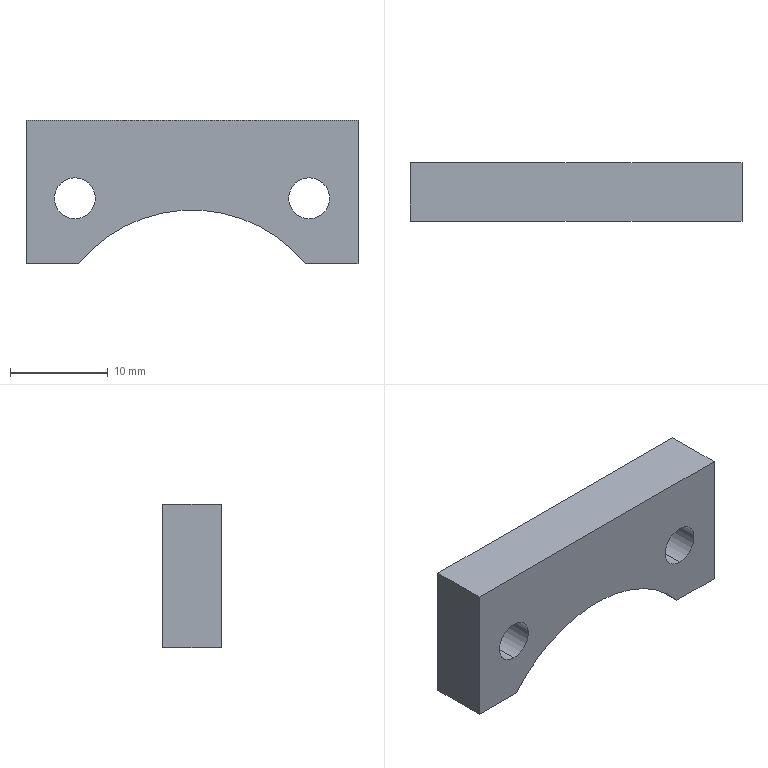Part | SolidWorks | features 3DProfileFeature 1, FlatPattern 1, HoleWzd 1, SMBaseFlange 1, SheetMetal 1 | 1 solid | 12 faces | box 34 x 6 x 14.7 mm | volume 2300 mm3 | plane 7 | cylinder 5 | commonest cylinder face diameters 4.2 x4 30 x1
STEP:
#1=CARTESIAN_POINT('',(-12.,0.,-2.75));
#2=VERTEX_POINT('',#1);
#3=CARTESIAN_POINT('',(-12.,0.,1.45));
#4=VERTEX_POINT('',#3);
#5=CARTESIAN_POINT('',(-12.,0.,-0.65));
#6=DIRECTION('',(0.,1.,0.));
#7=DIRECTION('',(0.,0.,1.));
#8=AXIS2_PLACEMENT_3D('',#5,#6,#7);
#9=CIRCLE('',#8,2.1);
#10=EDGE_CURVE('',#2,#4,#9,.T.);
#11=ORIENTED_EDGE('',*,*,#10,.F.);
#12=CARTESIAN_POINT('',(-12.,6.,-2.75));
#13=VERTEX_POINT('',#12);
#14=CARTESIAN_POINT('',(-12.,6.,-2.75));
#15=DIRECTION('',(0.,1.,0.));
#16=VECTOR('',#15,1000.);
#17=LINE('',#14,#16);
#18=EDGE_CURVE('',#2,#13,#17,.T.);
#19=ORIENTED_EDGE('',*,*,#18,.T.);
#20=CARTESIAN_POINT('',(-12.,6.,1.45));
#21=VERTEX_POINT('',#20);
#22=CARTESIAN_POINT('',(-12.,6.,-0.65));
#23=DIRECTION('',(0.,1.,0.));
#24=DIRECTION('',(0.,0.,1.));
#25=AXIS2_PLACEMENT_3D('',#22,#23,#24);
#26=CIRCLE('',#25,2.1);
#27=EDGE_CURVE('',#13,#21,#26,.T.);
#28=ORIENTED_EDGE('',*,*,#27,.T.);
#29=CARTESIAN_POINT('',(-12.,6.,1.45));
#30=DIRECTION('',(0.,1.,0.));
#31=VECTOR('',#30,1000.);
#32=LINE('',#29,#31);
#33=EDGE_CURVE('',#4,#21,#32,.T.);
#34=ORIENTED_EDGE('',*,*,#33,.F.);
#35=EDGE_LOOP('',(#11,#19,#28,#34));
#36=FACE_OUTER_BOUND('',#35,.T.);
#37=CARTESIAN_POINT('',(-12.,6.,-0.65));
#38=DIRECTION('',(0.,1.,0.));
#39=DIRECTION('',(0.,0.,1.));
#40=AXIS2_PLACEMENT_3D('',#37,#38,#39);
#41=CYLINDRICAL_SURFACE('',#40,2.1);
#42=ADVANCED_FACE('',(#36),#41,.F.);
#43=CARTESIAN_POINT('',(12.,0.,-2.75));
#44=VERTEX_POINT('',#43);
#45=CARTESIAN_POINT('',(12.,0.,1.45));
#46=VERTEX_POINT('',#45);
#47=CARTESIAN_POINT('',(12.,0.,-0.65));
#48=DIRECTION('',(0.,1.,0.));
#49=DIRECTION('',(0.,0.,1.));
#50=AXIS2_PLACEMENT_3D('',#47,#48,#49);
#51=CIRCLE('',#50,2.1);
#52=EDGE_CURVE('',#44,#46,#51,.T.);
#53=ORIENTED_EDGE('',*,*,#52,.F.);
#54=CARTESIAN_POINT('',(12.,6.,-2.75));
#55=VERTEX_POINT('',#54);
#56=CARTESIAN_POINT('',(12.,6.,-2.75));
#57=DIRECTION('',(0.,1.,0.));
#58=VECTOR('',#57,1000.);
#59=LINE('',#56,#58);
#60=EDGE_CURVE('',#44,#55,#59,.T.);
#61=ORIENTED_EDGE('',*,*,#60,.T.);
#62=CARTESIAN_POINT('',(12.,6.,1.45));
#63=VERTEX_POINT('',#62);
#64=CARTESIAN_POINT('',(12.,6.,-0.65));
#65=DIRECTION('',(0.,1.,0.));
#66=DIRECTION('',(0.,0.,1.));
#67=AXIS2_PLACEMENT_3D('',#64,#65,#66);
#68=CIRCLE('',#67,2.1);
#69=EDGE_CURVE('',#55,#63,#68,.T.);
#70=ORIENTED_EDGE('',*,*,#69,.T.);
#71=CARTESIAN_POINT('',(12.,6.,1.45));
#72=DIRECTION('',(0.,1.,0.));
#73=VECTOR('',#72,1000.);
#74=LINE('',#71,#73);
#75=EDGE_CURVE('',#46,#63,#74,.T.);
#76=ORIENTED_EDGE('',*,*,#75,.F.);
#77=EDGE_LOOP('',(#53,#61,#70,#76));
#78=FACE_OUTER_BOUND('',#77,.T.);
#79=CARTESIAN_POINT('',(12.,6.,-0.65));
#80=DIRECTION('',(0.,1.,0.));
#81=DIRECTION('',(0.,0.,1.));
#82=AXIS2_PLACEMENT_3D('',#79,#80,#81);
#83=CYLINDRICAL_SURFACE('',#82,2.1);
#84=ADVANCED_FACE('',(#78),#83,.F.);
#85=CARTESIAN_POINT('',(-12.,6.,-0.65));
#86=DIRECTION('',(0.,1.,0.));
#87=DIRECTION('',(0.,0.,1.));
#88=AXIS2_PLACEMENT_3D('',#85,#86,#87);
#89=CIRCLE('',#88,2.1);
#90=EDGE_CURVE('',#21,#13,#89,.T.);
#91=ORIENTED_EDGE('',*,*,#90,.F.);
#92=ORIENTED_EDGE('',*,*,#27,.F.);
#93=EDGE_LOOP('',(#91,#92));
#94=FACE_BOUND('',#93,.T.);
#95=CARTESIAN_POINT('',(12.,6.,-0.65));
#96=DIRECTION('',(0.,1.,0.));
#97=DIRECTION('',(0.,0.,1.));
#98=AXIS2_PLACEMENT_3D('',#95,#96,#97);
#99=CIRCLE('',#98,2.1);
#100=EDGE_CURVE('',#63,#55,#99,.T.);
#101=ORIENTED_EDGE('',*,*,#100,.F.);
#102=ORIENTED_EDGE('',*,*,#69,.F.);
#103=EDGE_LOOP('',(#101,#102));
#104=FACE_BOUND('',#103,.T.);
#105=CARTESIAN_POINT('',(17.,6.,7.35));
#106=VERTEX_POINT('',#105);
#107=CARTESIAN_POINT('',(17.,6.,-7.35));
#108=VERTEX_POINT('',#107);
#109=CARTESIAN_POINT('',(17.,6.,-7.35));
#110=DIRECTION('',(0.,0.,-1.));
#111=VECTOR('',#110,1000.);
#112=LINE('',#109,#111);
#113=EDGE_CURVE('',#106,#108,#112,.T.);
#114=ORIENTED_EDGE('',*,*,#113,.T.);
#115=CARTESIAN_POINT('',(11.608,6.,-7.35));
#116=VERTEX_POINT('',#115);
#117=CARTESIAN_POINT('',(11.608,6.,-7.35));
#118=DIRECTION('',(-1.,0.,0.));
#119=VECTOR('',#118,1000.);
#120=LINE('',#117,#119);
#121=EDGE_CURVE('',#108,#116,#120,.T.);
#122=ORIENTED_EDGE('',*,*,#121,.T.);
#123=CARTESIAN_POINT('',(-11.608,6.,-7.35));
#124=VERTEX_POINT('',#123);
#125=CARTESIAN_POINT('',(0.,6.,-16.85));
#126=DIRECTION('',(0.,-1.,0.));
#127=DIRECTION('',(0.,0.,1.));
#128=AXIS2_PLACEMENT_3D('',#125,#126,#127);
#129=CIRCLE('',#128,15.);
#130=EDGE_CURVE('',#116,#124,#129,.T.);
#131=ORIENTED_EDGE('',*,*,#130,.T.);
#132=CARTESIAN_POINT('',(-17.,6.,-7.35));
#133=VERTEX_POINT('',#132);
#134=CARTESIAN_POINT('',(-17.,6.,-7.35));
#135=DIRECTION('',(-1.,0.,0.));
#136=VECTOR('',#135,1000.);
#137=LINE('',#134,#136);
#138=EDGE_CURVE('',#124,#133,#137,.T.);
#139=ORIENTED_EDGE('',*,*,#138,.T.);
#140=CARTESIAN_POINT('',(-17.,6.,7.35));
#141=VERTEX_POINT('',#140);
#142=CARTESIAN_POINT('',(-17.,6.,-7.35));
#143=DIRECTION('',(0.,0.,1.));
#144=VECTOR('',#143,1000.);
#145=LINE('',#142,#144);
#146=EDGE_CURVE('',#133,#141,#145,.T.);
#147=ORIENTED_EDGE('',*,*,#146,.T.);
#148=CARTESIAN_POINT('',(-17.,6.,7.35));
#149=DIRECTION('',(1.,0.,0.));
#150=VECTOR('',#149,1000.);
#151=LINE('',#148,#150);
#152=EDGE_CURVE('',#141,#106,#151,.T.);
#153=ORIENTED_EDGE('',*,*,#152,.T.);
#154=EDGE_LOOP('',(#114,#122,#131,#139,#147,#153));
#155=FACE_OUTER_BOUND('',#154,.T.);
#156=CARTESIAN_POINT('',(0.,6.,-16.85));
#157=DIRECTION('',(0.,1.,0.));
#158=DIRECTION('',(0.,0.,1.));
#159=AXIS2_PLACEMENT_3D('',#156,#157,#158);
#160=PLANE('',#159);
#161=ADVANCED_FACE('',(#94,#104,#155),#160,.T.);
#162=CARTESIAN_POINT('',(-12.,0.,-0.65));
#163=DIRECTION('',(0.,1.,0.));
#164=DIRECTION('',(0.,0.,1.));
#165=AXIS2_PLACEMENT_3D('',#162,#163,#164);
#166=CIRCLE('',#165,2.1);
#167=EDGE_CURVE('',#4,#2,#166,.T.);
#168=ORIENTED_EDGE('',*,*,#167,.T.);
#169=ORIENTED_EDGE('',*,*,#10,.T.);
#170=EDGE_LOOP('',(#168,#169));
#171=FACE_BOUND('',#170,.T.);
#172=CARTESIAN_POINT('',(12.,0.,-0.65));
#173=DIRECTION('',(0.,1.,0.));
#174=DIRECTION('',(0.,0.,1.));
#175=AXIS2_PLACEMENT_3D('',#172,#173,#174);
#176=CIRCLE('',#175,2.1);
#177=EDGE_CURVE('',#46,#44,#176,.T.);
#178=ORIENTED_EDGE('',*,*,#177,.T.);
#179=ORIENTED_EDGE('',*,*,#52,.T.);
#180=EDGE_LOOP('',(#178,#179));
#181=FACE_BOUND('',#180,.T.);
#182=CARTESIAN_POINT('',(17.,0.,7.35));
#183=VERTEX_POINT('',#182);
#184=CARTESIAN_POINT('',(17.,0.,-7.35));
#185=VERTEX_POINT('',#184);
#186=CARTESIAN_POINT('',(17.,0.,-7.35));
#187=DIRECTION('',(0.,0.,-1.));
#188=VECTOR('',#187,1000.);
#189=LINE('',#186,#188);
#190=EDGE_CURVE('',#183,#185,#189,.T.);
#191=ORIENTED_EDGE('',*,*,#190,.F.);
#192=CARTESIAN_POINT('',(-17.,0.,7.35));
#193=VERTEX_POINT('',#192);
#194=CARTESIAN_POINT('',(-17.,0.,7.35));
#195=DIRECTION('',(1.,0.,0.));
#196=VECTOR('',#195,1000.);
#197=LINE('',#194,#196);
#198=EDGE_CURVE('',#193,#183,#197,.T.);
#199=ORIENTED_EDGE('',*,*,#198,.F.);
#200=CARTESIAN_POINT('',(-17.,0.,-7.35));
#201=VERTEX_POINT('',#200);
#202=CARTESIAN_POINT('',(-17.,0.,-7.35));
#203=DIRECTION('',(0.,0.,1.));
#204=VECTOR('',#203,1000.);
#205=LINE('',#202,#204);
#206=EDGE_CURVE('',#201,#193,#205,.T.);
#207=ORIENTED_EDGE('',*,*,#206,.F.);
#208=CARTESIAN_POINT('',(-11.608,0.,-7.35));
#209=VERTEX_POINT('',#208);
#210=CARTESIAN_POINT('',(-17.,0.,-7.35));
#211=DIRECTION('',(-1.,0.,0.));
#212=VECTOR('',#211,1000.);
#213=LINE('',#210,#212);
#214=EDGE_CURVE('',#209,#201,#213,.T.);
#215=ORIENTED_EDGE('',*,*,#214,.F.);
#216=CARTESIAN_POINT('',(11.608,0.,-7.35));
#217=VERTEX_POINT('',#216);
#218=CARTESIAN_POINT('',(0.,0.,-16.85));
#219=DIRECTION('',(0.,-1.,0.));
#220=DIRECTION('',(0.,0.,1.));
#221=AXIS2_PLACEMENT_3D('',#218,#219,#220);
#222=CIRCLE('',#221,15.);
#223=EDGE_CURVE('',#217,#209,#222,.T.);
#224=ORIENTED_EDGE('',*,*,#223,.F.);
#225=CARTESIAN_POINT('',(11.608,0.,-7.35));
#226=DIRECTION('',(-1.,0.,0.));
#227=VECTOR('',#226,1000.);
#228=LINE('',#225,#227);
#229=EDGE_CURVE('',#185,#217,#228,.T.);
#230=ORIENTED_EDGE('',*,*,#229,.F.);
#231=EDGE_LOOP('',(#191,#199,#207,#215,#224,#230));
#232=FACE_OUTER_BOUND('',#231,.T.);
#233=CARTESIAN_POINT('',(0.,0.,-16.85));
#234=DIRECTION('',(0.,1.,0.));
#235=DIRECTION('',(0.,0.,1.));
#236=AXIS2_PLACEMENT_3D('',#233,#234,#235);
#237=PLANE('',#236);
#238=ADVANCED_FACE('',(#171,#181,#232),#237,.F.);
#239=ORIENTED_EDGE('',*,*,#190,.T.);
#240=CARTESIAN_POINT('',(17.,6.,-7.35));
#241=DIRECTION('',(0.,-1.,0.));
#242=VECTOR('',#241,1000.);
#243=LINE('',#240,#242);
#244=EDGE_CURVE('',#108,#185,#243,.T.);
#245=ORIENTED_EDGE('',*,*,#244,.F.);
#246=ORIENTED_EDGE('',*,*,#113,.F.);
#247=CARTESIAN_POINT('',(17.,6.,7.35));
#248=DIRECTION('',(0.,-1.,0.));
#249=VECTOR('',#248,1000.);
#250=LINE('',#247,#249);
#251=EDGE_CURVE('',#106,#183,#250,.T.);
#252=ORIENTED_EDGE('',*,*,#251,.T.);
#253=EDGE_LOOP('',(#239,#245,#246,#252));
#254=FACE_OUTER_BOUND('',#253,.T.);
#255=CARTESIAN_POINT('',(17.,6.,-7.35));
#256=DIRECTION('',(-1.,0.,0.));
#257=DIRECTION('',(0.,0.,1.));
#258=AXIS2_PLACEMENT_3D('',#255,#256,#257);
#259=PLANE('',#258);
#260=ADVANCED_FACE('',(#254),#259,.F.);
#261=ORIENTED_EDGE('',*,*,#229,.T.);
#262=CARTESIAN_POINT('',(11.608,6.,-7.35));
#263=DIRECTION('',(0.,-1.,0.));
#264=VECTOR('',#263,1000.);
#265=LINE('',#262,#264);
#266=EDGE_CURVE('',#116,#217,#265,.T.);
#267=ORIENTED_EDGE('',*,*,#266,.F.);
#268=ORIENTED_EDGE('',*,*,#121,.F.);
#269=ORIENTED_EDGE('',*,*,#244,.T.);
#270=EDGE_LOOP('',(#261,#267,#268,#269));
#271=FACE_OUTER_BOUND('',#270,.T.);
#272=CARTESIAN_POINT('',(11.608,6.,-7.35));
#273=DIRECTION('',(0.,0.,1.));
#274=DIRECTION('',(1.,0.,0.));
#275=AXIS2_PLACEMENT_3D('',#272,#273,#274);
#276=PLANE('',#275);
#277=ADVANCED_FACE('',(#271),#276,.F.);
#278=ORIENTED_EDGE('',*,*,#223,.T.);
#279=CARTESIAN_POINT('',(-11.608,6.,-7.35));
#280=DIRECTION('',(0.,-1.,0.));
#281=VECTOR('',#280,1000.);
#282=LINE('',#279,#281);
#283=EDGE_CURVE('',#124,#209,#282,.T.);
#284=ORIENTED_EDGE('',*,*,#283,.F.);
#285=ORIENTED_EDGE('',*,*,#130,.F.);
#286=ORIENTED_EDGE('',*,*,#266,.T.);
#287=EDGE_LOOP('',(#278,#284,#285,#286));
#288=FACE_OUTER_BOUND('',#287,.T.);
#289=CARTESIAN_POINT('',(0.,6.,-16.85));
#290=DIRECTION('',(0.,-1.,0.));
#291=DIRECTION('',(0.,0.,-1.));
#292=AXIS2_PLACEMENT_3D('',#289,#290,#291);
#293=CYLINDRICAL_SURFACE('',#292,15.);
#294=ADVANCED_FACE('',(#288),#293,.F.);
#295=ORIENTED_EDGE('',*,*,#214,.T.);
#296=CARTESIAN_POINT('',(-17.,6.,-7.35));
#297=DIRECTION('',(0.,-1.,0.));
#298=VECTOR('',#297,1000.);
#299=LINE('',#296,#298);
#300=EDGE_CURVE('',#133,#201,#299,.T.);
#301=ORIENTED_EDGE('',*,*,#300,.F.);
#302=ORIENTED_EDGE('',*,*,#138,.F.);
#303=ORIENTED_EDGE('',*,*,#283,.T.);
#304=EDGE_LOOP('',(#295,#301,#302,#303));
#305=FACE_OUTER_BOUND('',#304,.T.);
#306=CARTESIAN_POINT('',(-17.,6.,-7.35));
#307=DIRECTION('',(0.,0.,1.));
#308=DIRECTION('',(1.,0.,0.));
#309=AXIS2_PLACEMENT_3D('',#306,#307,#308);
#310=PLANE('',#309);
#311=ADVANCED_FACE('',(#305),#310,.F.);
#312=ORIENTED_EDGE('',*,*,#206,.T.);
#313=CARTESIAN_POINT('',(-17.,6.,7.35));
#314=DIRECTION('',(0.,-1.,0.));
#315=VECTOR('',#314,1000.);
#316=LINE('',#313,#315);
#317=EDGE_CURVE('',#141,#193,#316,.T.);
#318=ORIENTED_EDGE('',*,*,#317,.F.);
#319=ORIENTED_EDGE('',*,*,#146,.F.);
#320=ORIENTED_EDGE('',*,*,#300,.T.);
#321=EDGE_LOOP('',(#312,#318,#319,#320));
#322=FACE_OUTER_BOUND('',#321,.T.);
#323=CARTESIAN_POINT('',(-17.,6.,-7.35));
#324=DIRECTION('',(1.,0.,0.));
#325=DIRECTION('',(0.,0.,-1.));
#326=AXIS2_PLACEMENT_3D('',#323,#324,#325);
#327=PLANE('',#326);
#328=ADVANCED_FACE('',(#322),#327,.F.);
#329=ORIENTED_EDGE('',*,*,#198,.T.);
#330=ORIENTED_EDGE('',*,*,#251,.F.);
#331=ORIENTED_EDGE('',*,*,#152,.F.);
#332=ORIENTED_EDGE('',*,*,#317,.T.);
#333=EDGE_LOOP('',(#329,#330,#331,#332));
#334=FACE_OUTER_BOUND('',#333,.T.);
#335=CARTESIAN_POINT('',(-17.,6.,7.35));
#336=DIRECTION('',(0.,0.,-1.));
#337=DIRECTION('',(-1.,0.,0.));
#338=AXIS2_PLACEMENT_3D('',#335,#336,#337);
#339=PLANE('',#338);
#340=ADVANCED_FACE('',(#334),#339,.F.);
#341=ORIENTED_EDGE('',*,*,#60,.F.);
#342=ORIENTED_EDGE('',*,*,#177,.F.);
#343=ORIENTED_EDGE('',*,*,#75,.T.);
#344=ORIENTED_EDGE('',*,*,#100,.T.);
#345=EDGE_LOOP('',(#341,#342,#343,#344));
#346=FACE_OUTER_BOUND('',#345,.T.);
#347=CARTESIAN_POINT('',(12.,6.,-0.65));
#348=DIRECTION('',(0.,1.,0.));
#349=DIRECTION('',(0.,0.,1.));
#350=AXIS2_PLACEMENT_3D('',#347,#348,#349);
#351=CYLINDRICAL_SURFACE('',#350,2.1);
#352=ADVANCED_FACE('',(#346),#351,.F.);
#353=ORIENTED_EDGE('',*,*,#18,.F.);
#354=ORIENTED_EDGE('',*,*,#167,.F.);
#355=ORIENTED_EDGE('',*,*,#33,.T.);
#356=ORIENTED_EDGE('',*,*,#90,.T.);
#357=EDGE_LOOP('',(#353,#354,#355,#356));
#358=FACE_OUTER_BOUND('',#357,.T.);
#359=CARTESIAN_POINT('',(-12.,6.,-0.65));
#360=DIRECTION('',(0.,1.,0.));
#361=DIRECTION('',(0.,0.,1.));
#362=AXIS2_PLACEMENT_3D('',#359,#360,#361);
#363=CYLINDRICAL_SURFACE('',#362,2.1);
#364=ADVANCED_FACE('',(#358),#363,.F.);
#365=CLOSED_SHELL('',(#42,#84,#161,#238,#260,#277,#294,#311,#328,#340,#352,#364));
#366=MANIFOLD_SOLID_BREP('',#365);
#367=CARTESIAN_POINT('',(0.,0.,0.));
#368=DIRECTION('',(0.,0.,1.));
#369=DIRECTION('',(1.,0.,0.));
#370=AXIS2_PLACEMENT_3D('',#367,#368,#369);
#371=(LENGTH_UNIT()NAMED_UNIT(*)SI_UNIT(.MILLI.,.METRE.));
#372=UNCERTAINTY_MEASURE_WITH_UNIT(LENGTH_MEASURE(0.00001),#371,'','');
#373=(NAMED_UNIT(*)PLANE_ANGLE_UNIT()SI_UNIT($,.RADIAN.));
#374=(NAMED_UNIT(*)SI_UNIT($,.STERADIAN.)SOLID_ANGLE_UNIT());
#375=(GEOMETRIC_REPRESENTATION_CONTEXT(3)GLOBAL_UNCERTAINTY_ASSIGNED_CONTEXT((#372))GLOBAL_UNIT_ASSIGNED_CONTEXT((#371,#373,#374))REPRESENTATION_CONTEXT('',''));
#376=ADVANCED_BREP_SHAPE_REPRESENTATION('',(#366,#370),#375);